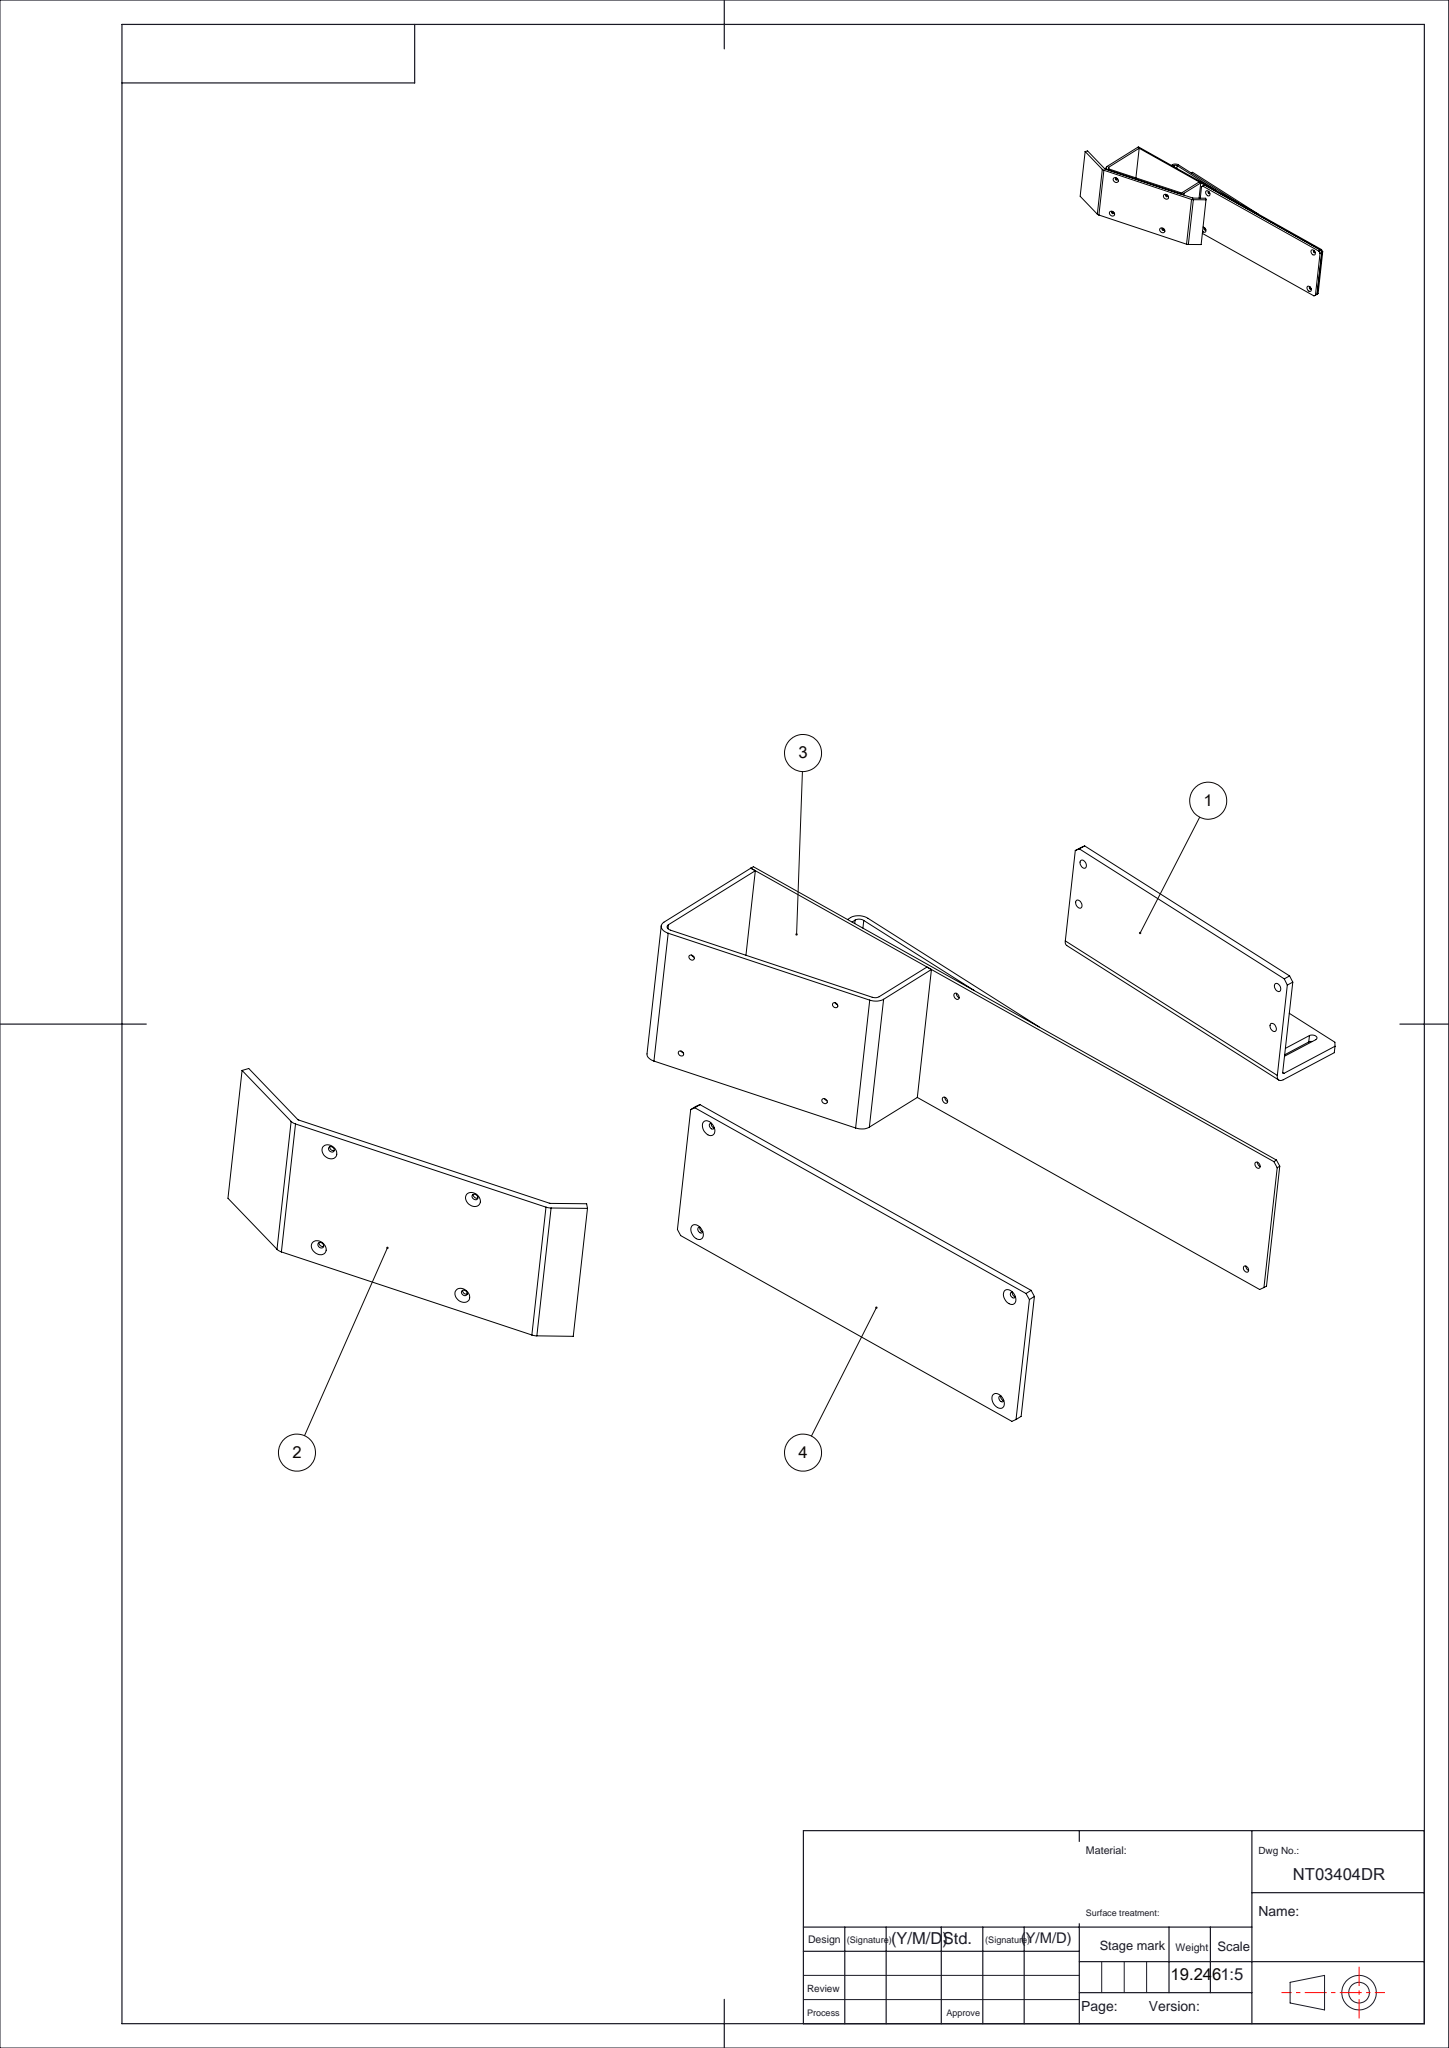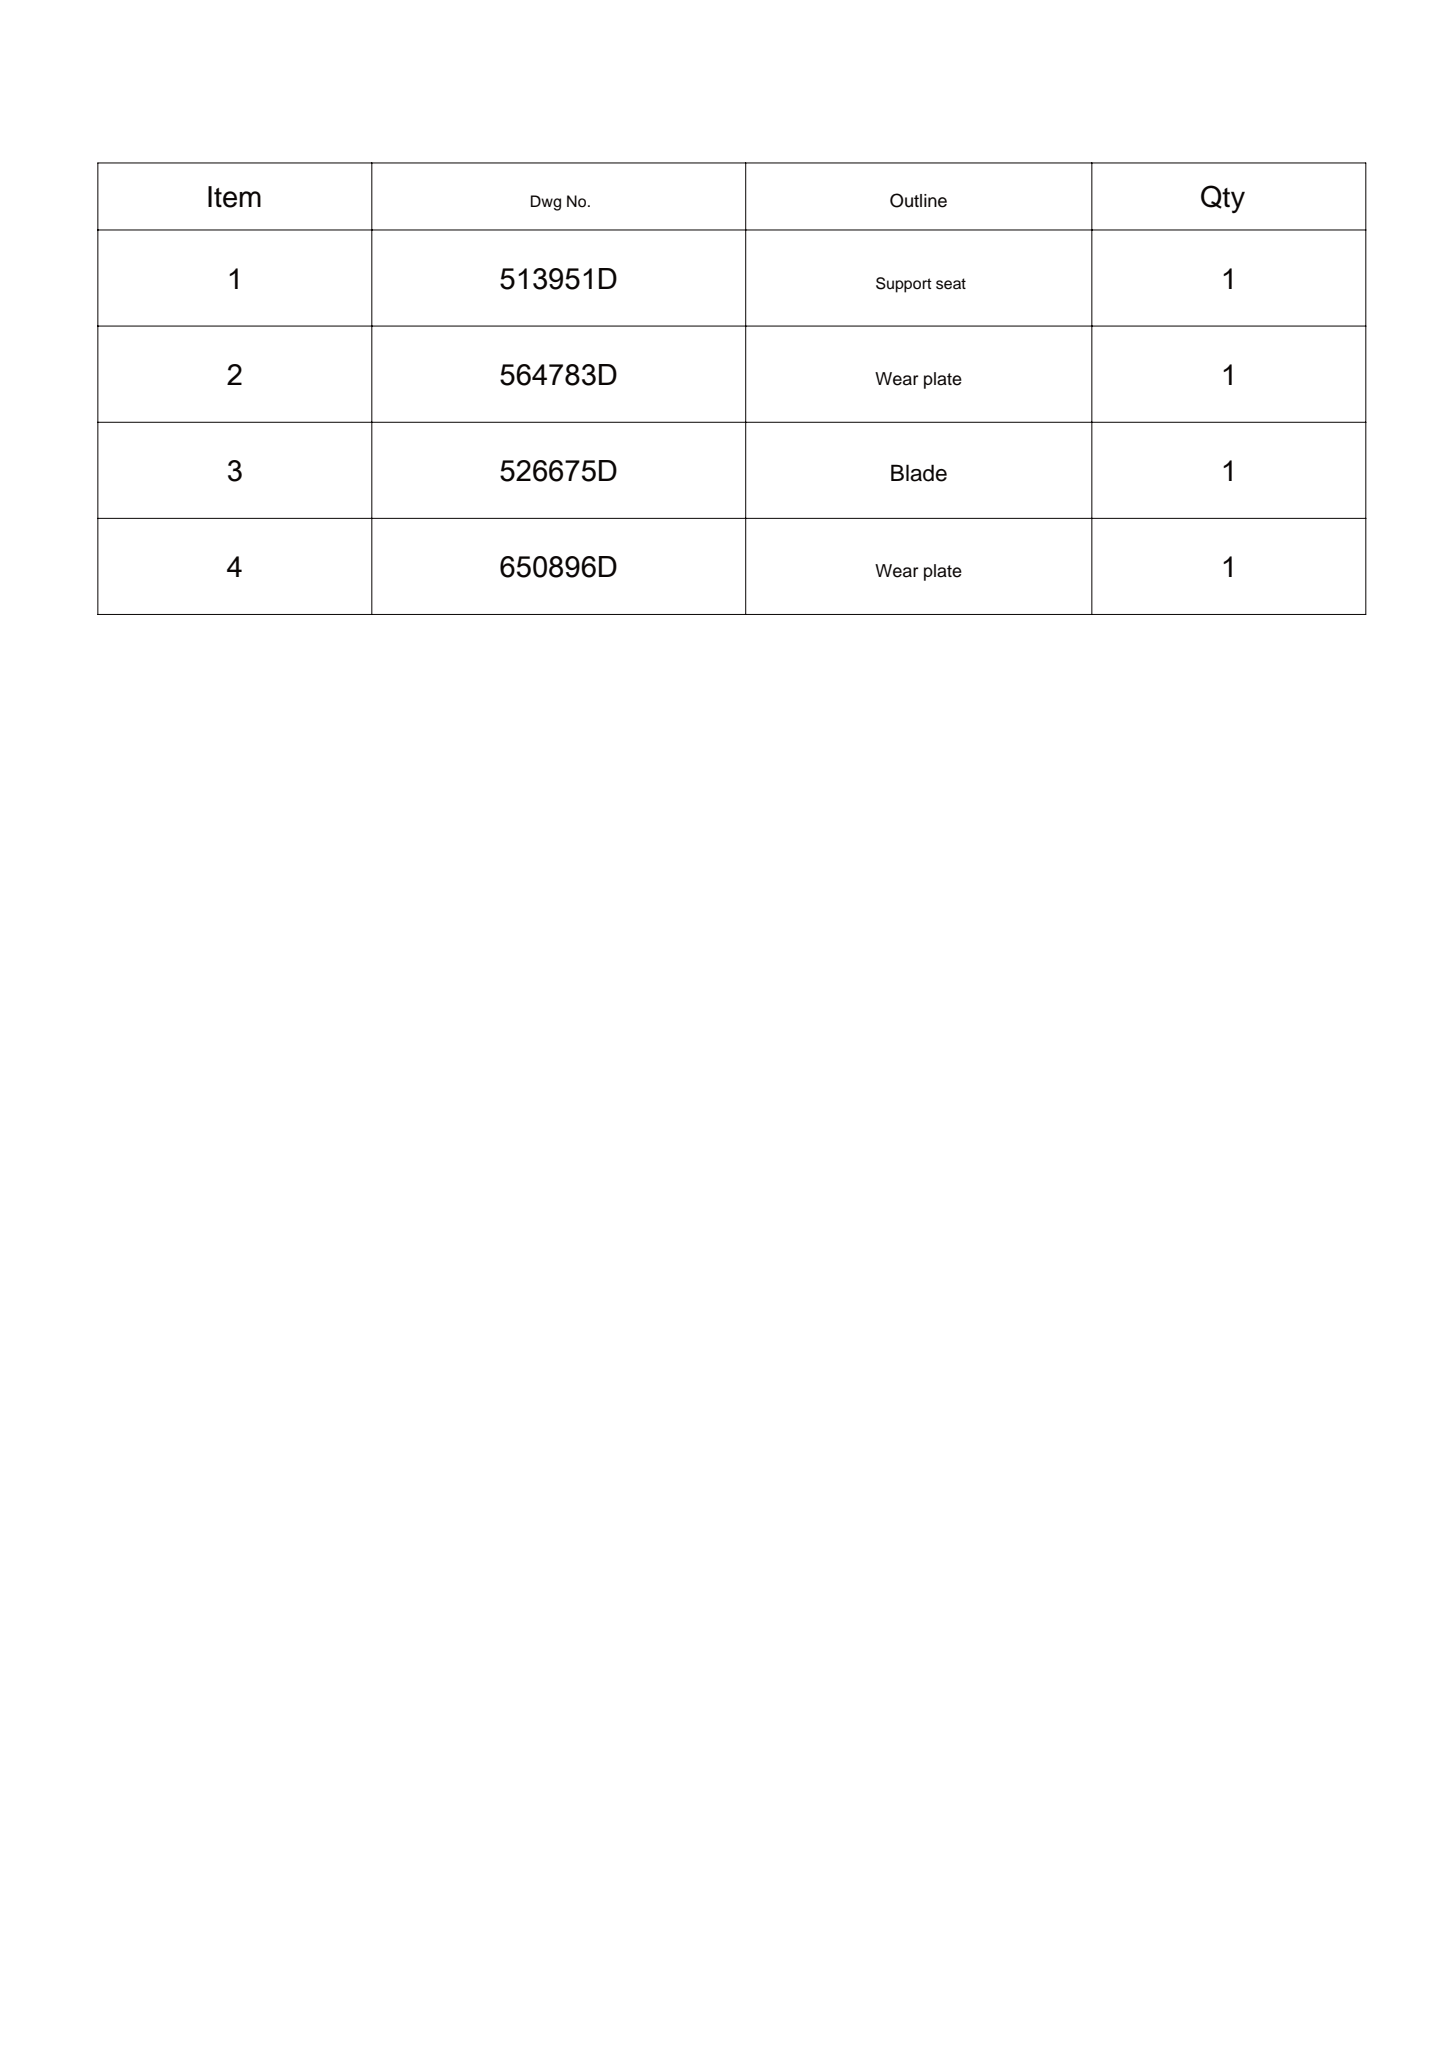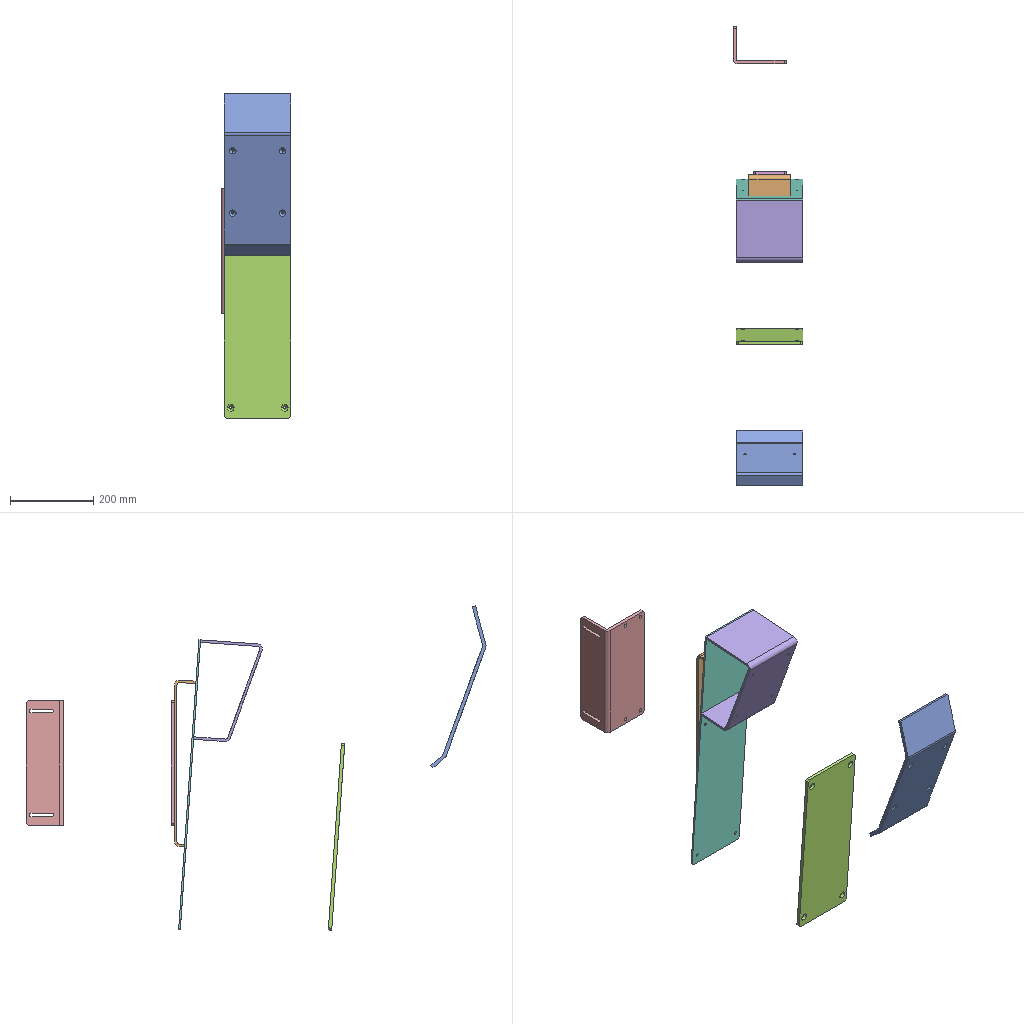Assembly | SolidWorks | 8 different items | 8 placed | box 168 x 1107 x 781 mm
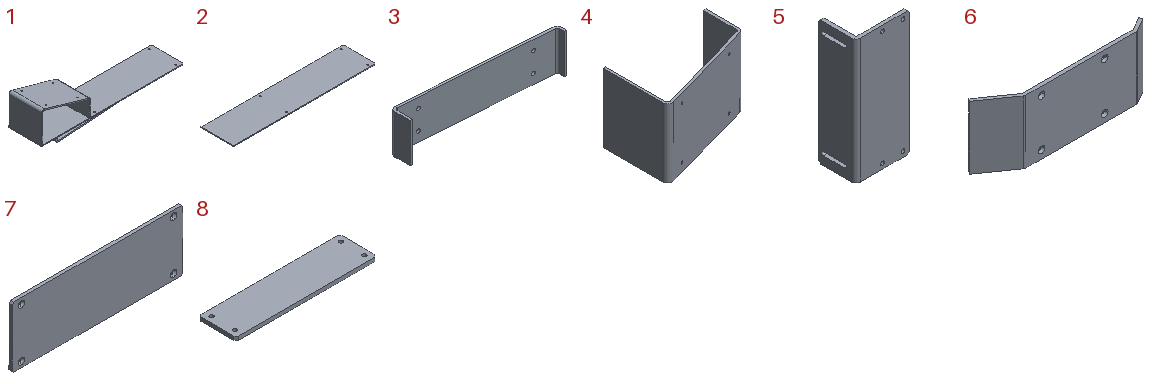Parts list (item | name | quantity | parent item | size | volume | features):
1 | (subassembly) | x1 | - | 700 x 160 x 210.348 mm | 1357509 mm3 | features CompositeCurve 4
2 | - | x1 | in 1 | 700 x 160 x 4 mm | 447284 mm3 | features Chamfer 1, Extrusion 1, ICE 1
3 | - | x1 | in 1 | 400 x 51.131 x 100 mm | 272755 mm3 | features Fillet 2, Extrusion 1, ICE 1
4 | - | x1 | in 1 | 240 x 149.894 x 160 mm | 447479 mm3 | features Extrusion 1, ICE 1
5 | - | x1 | - | 128 x 90 x 300 mm | 487166 mm3 | features Fillet 2, ICE 2, Chamfer 1, Extrusion 1
6 | - | x1 | - | 401.556 x 63.911 x 160 mm | 535175 mm3 | features Fillet 2, ICE 2, Extrusion 1
7 | - | x1 | - | 450 x 8 x 160 mm | 572994 mm3 | features ICE 2, Chamfer 1, Extrusion 1
8 | - | x1 | in 1 | 300 x 80 x 8 mm | 189992 mm3 | features Chamfer 1, Extrusion 1, ICE 1
Mates (type | each side: item.copy, entity, surface, feature):
In the top assembly
Coincident | 5.1 face plane Boss-Extrude1 | 8.1 face plane Boss-Extrude1
Concentric | 5.1 face cylinder Cut-Extrude1 | 8.1 edge
Concentric | 5.1 edge | 8.1 edge
Coincident | 6.1 face plane Boss-Extrude4 | 4.1 face plane Boss-Extrude1
Concentric | 6.1 edge | 4.1 edge | 2 times
Coincident | 7.1 face plane Boss-Extrude1 | 2.1 face plane Boss-Extrude1
Concentric | 7.1 edge | 2.1 edge | 2 times
In subassembly 1
Concentric | 8.2 edge | 3.1 edge | 2 times
Coincident | 2.2 face plane Boss-Extrude1 | 3.1 face plane Boss-Extrude1
Width | 3.1 face plane Boss-Extrude1 | 3.1 face plane Boss-Extrude1 | 2.2 face plane Boss-Extrude1 | 2.2 face plane Boss-Extrude1
Coincident | 2.2 face plane Boss-Extrude1 | 4.2 face plane Boss-Extrude1 | 3 times
DistanceDim | 3.1 face plane Boss-Extrude1 | 2.2 face plane Boss-Extrude1
Coincident | 2.2 face plane Boss-Extrude1 | 1.1 plane